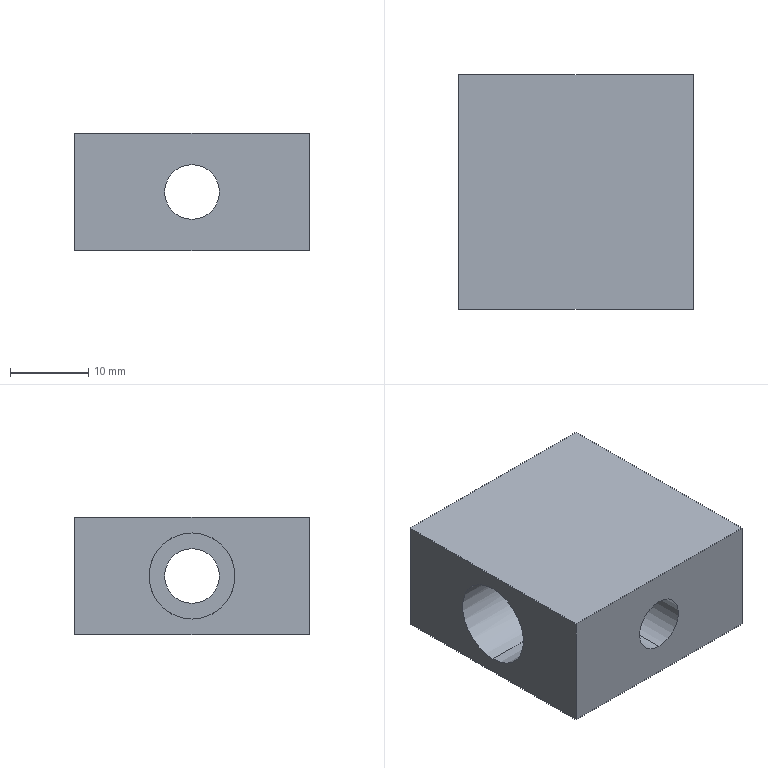Part | SolidWorks | features BaseBody 1 | 1 solid | 20 faces | box 30 x 30 x 15 mm | volume 9251 mm3 | cylinder 12 | plane 8 | commonest cylinder face diameters 11 x8 7 x4
STEP:
#1=CARTESIAN_POINT('',(30.,15.,4.));
#2=VERTEX_POINT('',#1);
#3=CARTESIAN_POINT('',(30.,15.,11.));
#4=VERTEX_POINT('',#3);
#5=CARTESIAN_POINT('',(30.,15.,7.5));
#6=DIRECTION('',(-1.,0.,0.));
#7=DIRECTION('',(0.,0.,1.));
#8=AXIS2_PLACEMENT_3D('',#5,#6,#7);
#9=CIRCLE('',#8,3.5);
#10=EDGE_CURVE('',#2,#4,#9,.T.);
#11=ORIENTED_EDGE('',*,*,#10,.F.);
#12=CARTESIAN_POINT('',(25.,15.,4.));
#13=VERTEX_POINT('',#12);
#14=CARTESIAN_POINT('',(0.,15.,4.));
#15=DIRECTION('',(-1.,0.,0.));
#16=VECTOR('',#15,1000.);
#17=LINE('',#14,#16);
#18=EDGE_CURVE('',#2,#13,#17,.T.);
#19=ORIENTED_EDGE('',*,*,#18,.T.);
#20=CARTESIAN_POINT('',(25.,15.,11.));
#21=VERTEX_POINT('',#20);
#22=CARTESIAN_POINT('',(25.,15.,7.5));
#23=DIRECTION('',(-1.,0.,0.));
#24=DIRECTION('',(0.,0.,1.));
#25=AXIS2_PLACEMENT_3D('',#22,#23,#24);
#26=CIRCLE('',#25,3.5);
#27=EDGE_CURVE('',#13,#21,#26,.T.);
#28=ORIENTED_EDGE('',*,*,#27,.T.);
#29=CARTESIAN_POINT('',(0.,15.,11.));
#30=DIRECTION('',(-1.,0.,0.));
#31=VECTOR('',#30,1000.);
#32=LINE('',#29,#31);
#33=EDGE_CURVE('',#4,#21,#32,.T.);
#34=ORIENTED_EDGE('',*,*,#33,.F.);
#35=EDGE_LOOP('',(#11,#19,#28,#34));
#36=FACE_OUTER_BOUND('',#35,.T.);
#37=CARTESIAN_POINT('',(0.,15.,7.5));
#38=DIRECTION('',(-1.,0.,0.));
#39=DIRECTION('',(0.,0.,1.));
#40=AXIS2_PLACEMENT_3D('',#37,#38,#39);
#41=CYLINDRICAL_SURFACE('',#40,3.5);
#42=ADVANCED_FACE('',(#36),#41,.F.);
#43=CARTESIAN_POINT('',(25.,15.,2.));
#44=VERTEX_POINT('',#43);
#45=CARTESIAN_POINT('',(25.,15.,13.));
#46=VERTEX_POINT('',#45);
#47=CARTESIAN_POINT('',(25.,15.,7.5));
#48=DIRECTION('',(-1.,0.,0.));
#49=DIRECTION('',(0.,0.,1.));
#50=AXIS2_PLACEMENT_3D('',#47,#48,#49);
#51=CIRCLE('',#50,5.5);
#52=EDGE_CURVE('',#44,#46,#51,.T.);
#53=ORIENTED_EDGE('',*,*,#52,.F.);
#54=CARTESIAN_POINT('',(15.,15.,2.));
#55=VERTEX_POINT('',#54);
#56=CARTESIAN_POINT('',(0.,15.,2.));
#57=DIRECTION('',(-1.,0.,0.));
#58=VECTOR('',#57,1000.);
#59=LINE('',#56,#58);
#60=EDGE_CURVE('',#44,#55,#59,.T.);
#61=ORIENTED_EDGE('',*,*,#60,.T.);
#62=CARTESIAN_POINT('',(15.,15.,13.));
#63=VERTEX_POINT('',#62);
#64=CARTESIAN_POINT('',(15.,15.,13.));
#65=CARTESIAN_POINT('',(26.,4.,13.));
#66=CARTESIAN_POINT('',(26.,4.,2.));
#67=CARTESIAN_POINT('',(15.,15.,2.));
#68=(BOUNDED_CURVE()B_SPLINE_CURVE(3,(#64,#65,#66,#67),.UNSPECIFIED.,.F.,.F.)B_SPLINE_CURVE_WITH_KNOTS((4,4),(1.571,4.712),.UNSPECIFIED.)CURVE()GEOMETRIC_REPRESENTATION_ITEM()RATIONAL_B_SPLINE_CURVE((1.,0.3333,0.3333,1.))REPRESENTATION_ITEM(''));
#69=EDGE_CURVE('',#63,#55,#68,.T.);
#70=ORIENTED_EDGE('',*,*,#69,.F.);
#71=CARTESIAN_POINT('',(0.,15.,13.));
#72=DIRECTION('',(-1.,0.,0.));
#73=VECTOR('',#72,1000.);
#74=LINE('',#71,#73);
#75=EDGE_CURVE('',#46,#63,#74,.T.);
#76=ORIENTED_EDGE('',*,*,#75,.F.);
#77=EDGE_LOOP('',(#53,#61,#70,#76));
#78=FACE_OUTER_BOUND('',#77,.T.);
#79=CARTESIAN_POINT('',(0.,15.,7.5));
#80=DIRECTION('',(-1.,0.,0.));
#81=DIRECTION('',(0.,0.,1.));
#82=AXIS2_PLACEMENT_3D('',#79,#80,#81);
#83=CYLINDRICAL_SURFACE('',#82,5.5);
#84=ADVANCED_FACE('',(#78),#83,.F.);
#85=CARTESIAN_POINT('',(15.,15.,2.));
#86=CARTESIAN_POINT('',(4.,4.,2.));
#87=CARTESIAN_POINT('',(4.,4.,13.));
#88=CARTESIAN_POINT('',(15.,15.,13.));
#89=(BOUNDED_CURVE()B_SPLINE_CURVE(3,(#85,#86,#87,#88),.UNSPECIFIED.,.F.,.F.)B_SPLINE_CURVE_WITH_KNOTS((4,4),(1.571,4.712),.UNSPECIFIED.)CURVE()GEOMETRIC_REPRESENTATION_ITEM()RATIONAL_B_SPLINE_CURVE((1.,0.3333,0.3333,1.))REPRESENTATION_ITEM(''));
#90=EDGE_CURVE('',#55,#63,#89,.T.);
#91=ORIENTED_EDGE('',*,*,#90,.F.);
#92=CARTESIAN_POINT('',(0.,15.,2.));
#93=VERTEX_POINT('',#92);
#94=CARTESIAN_POINT('',(0.,15.,2.));
#95=DIRECTION('',(-1.,0.,0.));
#96=VECTOR('',#95,1000.);
#97=LINE('',#94,#96);
#98=EDGE_CURVE('',#55,#93,#97,.T.);
#99=ORIENTED_EDGE('',*,*,#98,.T.);
#100=CARTESIAN_POINT('',(0.,15.,13.));
#101=VERTEX_POINT('',#100);
#102=CARTESIAN_POINT('',(0.,15.,7.5));
#103=DIRECTION('',(-1.,0.,0.));
#104=DIRECTION('',(0.,0.,1.));
#105=AXIS2_PLACEMENT_3D('',#102,#103,#104);
#106=CIRCLE('',#105,5.5);
#107=EDGE_CURVE('',#93,#101,#106,.T.);
#108=ORIENTED_EDGE('',*,*,#107,.T.);
#109=CARTESIAN_POINT('',(0.,15.,13.));
#110=DIRECTION('',(-1.,0.,0.));
#111=VECTOR('',#110,1000.);
#112=LINE('',#109,#111);
#113=EDGE_CURVE('',#63,#101,#112,.T.);
#114=ORIENTED_EDGE('',*,*,#113,.F.);
#115=EDGE_LOOP('',(#91,#99,#108,#114));
#116=FACE_OUTER_BOUND('',#115,.T.);
#117=CARTESIAN_POINT('',(0.,15.,7.5));
#118=DIRECTION('',(-1.,0.,0.));
#119=DIRECTION('',(0.,0.,1.));
#120=AXIS2_PLACEMENT_3D('',#117,#118,#119);
#121=CYLINDRICAL_SURFACE('',#120,5.5);
#122=ADVANCED_FACE('',(#116),#121,.F.);
#123=CARTESIAN_POINT('',(15.,5.,2.));
#124=VERTEX_POINT('',#123);
#125=CARTESIAN_POINT('',(15.,5.,13.));
#126=VERTEX_POINT('',#125);
#127=CARTESIAN_POINT('',(15.,5.,7.5));
#128=DIRECTION('',(0.,1.,0.));
#129=DIRECTION('',(0.,0.,1.));
#130=AXIS2_PLACEMENT_3D('',#127,#128,#129);
#131=CIRCLE('',#130,5.5);
#132=EDGE_CURVE('',#124,#126,#131,.T.);
#133=ORIENTED_EDGE('',*,*,#132,.F.);
#134=CARTESIAN_POINT('',(15.,30.,2.));
#135=DIRECTION('',(0.,1.,0.));
#136=VECTOR('',#135,1000.);
#137=LINE('',#134,#136);
#138=EDGE_CURVE('',#124,#55,#137,.T.);
#139=ORIENTED_EDGE('',*,*,#138,.T.);
#140=ORIENTED_EDGE('',*,*,#90,.T.);
#141=CARTESIAN_POINT('',(15.,30.,13.));
#142=DIRECTION('',(0.,1.,0.));
#143=VECTOR('',#142,1000.);
#144=LINE('',#141,#143);
#145=EDGE_CURVE('',#126,#63,#144,.T.);
#146=ORIENTED_EDGE('',*,*,#145,.F.);
#147=EDGE_LOOP('',(#133,#139,#140,#146));
#148=FACE_OUTER_BOUND('',#147,.T.);
#149=CARTESIAN_POINT('',(15.,30.,7.5));
#150=DIRECTION('',(0.,1.,0.));
#151=DIRECTION('',(0.,0.,1.));
#152=AXIS2_PLACEMENT_3D('',#149,#150,#151);
#153=CYLINDRICAL_SURFACE('',#152,5.5);
#154=ADVANCED_FACE('',(#148),#153,.F.);
#155=CARTESIAN_POINT('',(15.,0.,4.));
#156=VERTEX_POINT('',#155);
#157=CARTESIAN_POINT('',(15.,0.,11.));
#158=VERTEX_POINT('',#157);
#159=CARTESIAN_POINT('',(15.,0.,7.5));
#160=DIRECTION('',(0.,1.,0.));
#161=DIRECTION('',(0.,0.,1.));
#162=AXIS2_PLACEMENT_3D('',#159,#160,#161);
#163=CIRCLE('',#162,3.5);
#164=EDGE_CURVE('',#156,#158,#163,.T.);
#165=ORIENTED_EDGE('',*,*,#164,.F.);
#166=CARTESIAN_POINT('',(15.,5.,4.));
#167=VERTEX_POINT('',#166);
#168=CARTESIAN_POINT('',(15.,30.,4.));
#169=DIRECTION('',(0.,1.,0.));
#170=VECTOR('',#169,1000.);
#171=LINE('',#168,#170);
#172=EDGE_CURVE('',#156,#167,#171,.T.);
#173=ORIENTED_EDGE('',*,*,#172,.T.);
#174=CARTESIAN_POINT('',(15.,5.,11.));
#175=VERTEX_POINT('',#174);
#176=CARTESIAN_POINT('',(15.,5.,7.5));
#177=DIRECTION('',(0.,1.,0.));
#178=DIRECTION('',(0.,0.,1.));
#179=AXIS2_PLACEMENT_3D('',#176,#177,#178);
#180=CIRCLE('',#179,3.5);
#181=EDGE_CURVE('',#167,#175,#180,.T.);
#182=ORIENTED_EDGE('',*,*,#181,.T.);
#183=CARTESIAN_POINT('',(15.,30.,11.));
#184=DIRECTION('',(0.,1.,0.));
#185=VECTOR('',#184,1000.);
#186=LINE('',#183,#185);
#187=EDGE_CURVE('',#158,#175,#186,.T.);
#188=ORIENTED_EDGE('',*,*,#187,.F.);
#189=EDGE_LOOP('',(#165,#173,#182,#188));
#190=FACE_OUTER_BOUND('',#189,.T.);
#191=CARTESIAN_POINT('',(15.,30.,7.5));
#192=DIRECTION('',(0.,1.,0.));
#193=DIRECTION('',(0.,0.,1.));
#194=AXIS2_PLACEMENT_3D('',#191,#192,#193);
#195=CYLINDRICAL_SURFACE('',#194,3.5);
#196=ADVANCED_FACE('',(#190),#195,.F.);
#197=CARTESIAN_POINT('',(15.,15.,13.));
#198=CARTESIAN_POINT('',(4.,26.,13.));
#199=CARTESIAN_POINT('',(4.,26.,2.));
#200=CARTESIAN_POINT('',(15.,15.,2.));
#201=(BOUNDED_CURVE()B_SPLINE_CURVE(3,(#197,#198,#199,#200),.UNSPECIFIED.,.F.,.F.)B_SPLINE_CURVE_WITH_KNOTS((4,4),(4.712,7.854),.UNSPECIFIED.)CURVE()GEOMETRIC_REPRESENTATION_ITEM()RATIONAL_B_SPLINE_CURVE((1.,0.3333,0.3333,1.))REPRESENTATION_ITEM(''));
#202=EDGE_CURVE('',#63,#55,#201,.T.);
#203=ORIENTED_EDGE('',*,*,#202,.T.);
#204=CARTESIAN_POINT('',(15.,30.,2.));
#205=VERTEX_POINT('',#204);
#206=CARTESIAN_POINT('',(15.,30.,2.));
#207=DIRECTION('',(0.,1.,0.));
#208=VECTOR('',#207,1000.);
#209=LINE('',#206,#208);
#210=EDGE_CURVE('',#55,#205,#209,.T.);
#211=ORIENTED_EDGE('',*,*,#210,.T.);
#212=CARTESIAN_POINT('',(15.,30.,13.));
#213=VERTEX_POINT('',#212);
#214=CARTESIAN_POINT('',(15.,30.,7.5));
#215=DIRECTION('',(0.,1.,0.));
#216=DIRECTION('',(0.,0.,1.));
#217=AXIS2_PLACEMENT_3D('',#214,#215,#216);
#218=CIRCLE('',#217,5.5);
#219=EDGE_CURVE('',#205,#213,#218,.T.);
#220=ORIENTED_EDGE('',*,*,#219,.T.);
#221=CARTESIAN_POINT('',(15.,30.,13.));
#222=DIRECTION('',(0.,1.,0.));
#223=VECTOR('',#222,1000.);
#224=LINE('',#221,#223);
#225=EDGE_CURVE('',#63,#213,#224,.T.);
#226=ORIENTED_EDGE('',*,*,#225,.F.);
#227=EDGE_LOOP('',(#203,#211,#220,#226));
#228=FACE_OUTER_BOUND('',#227,.T.);
#229=CARTESIAN_POINT('',(15.,30.,7.5));
#230=DIRECTION('',(0.,1.,0.));
#231=DIRECTION('',(0.,0.,1.));
#232=AXIS2_PLACEMENT_3D('',#229,#230,#231);
#233=CYLINDRICAL_SURFACE('',#232,5.5);
#234=ADVANCED_FACE('',(#228),#233,.F.);
#235=CARTESIAN_POINT('',(25.,15.,7.5));
#236=DIRECTION('',(-1.,0.,0.));
#237=DIRECTION('',(0.,0.,1.));
#238=AXIS2_PLACEMENT_3D('',#235,#236,#237);
#239=CIRCLE('',#238,3.5);
#240=EDGE_CURVE('',#21,#13,#239,.T.);
#241=ORIENTED_EDGE('',*,*,#240,.F.);
#242=ORIENTED_EDGE('',*,*,#27,.F.);
#243=EDGE_LOOP('',(#241,#242));
#244=FACE_BOUND('',#243,.T.);
#245=CARTESIAN_POINT('',(25.,15.,7.5));
#246=DIRECTION('',(-1.,0.,0.));
#247=DIRECTION('',(0.,0.,1.));
#248=AXIS2_PLACEMENT_3D('',#245,#246,#247);
#249=CIRCLE('',#248,5.5);
#250=EDGE_CURVE('',#46,#44,#249,.T.);
#251=ORIENTED_EDGE('',*,*,#250,.T.);
#252=ORIENTED_EDGE('',*,*,#52,.T.);
#253=EDGE_LOOP('',(#251,#252));
#254=FACE_OUTER_BOUND('',#253,.T.);
#255=CARTESIAN_POINT('',(25.,18.5,7.5));
#256=DIRECTION('',(1.,0.,0.));
#257=DIRECTION('',(0.,1.,0.));
#258=AXIS2_PLACEMENT_3D('',#255,#256,#257);
#259=PLANE('',#258);
#260=ADVANCED_FACE('',(#244,#254),#259,.F.);
#261=CARTESIAN_POINT('',(15.,5.,7.5));
#262=DIRECTION('',(0.,1.,0.));
#263=DIRECTION('',(0.,0.,1.));
#264=AXIS2_PLACEMENT_3D('',#261,#262,#263);
#265=CIRCLE('',#264,3.5);
#266=EDGE_CURVE('',#175,#167,#265,.T.);
#267=ORIENTED_EDGE('',*,*,#266,.F.);
#268=ORIENTED_EDGE('',*,*,#181,.F.);
#269=EDGE_LOOP('',(#267,#268));
#270=FACE_BOUND('',#269,.T.);
#271=CARTESIAN_POINT('',(15.,5.,7.5));
#272=DIRECTION('',(0.,1.,0.));
#273=DIRECTION('',(0.,0.,1.));
#274=AXIS2_PLACEMENT_3D('',#271,#272,#273);
#275=CIRCLE('',#274,5.5);
#276=EDGE_CURVE('',#126,#124,#275,.T.);
#277=ORIENTED_EDGE('',*,*,#276,.T.);
#278=ORIENTED_EDGE('',*,*,#132,.T.);
#279=EDGE_LOOP('',(#277,#278));
#280=FACE_OUTER_BOUND('',#279,.T.);
#281=CARTESIAN_POINT('',(18.5,5.,7.5));
#282=DIRECTION('',(0.,-1.,0.));
#283=DIRECTION('',(0.,0.,-1.));
#284=AXIS2_PLACEMENT_3D('',#281,#282,#283);
#285=PLANE('',#284);
#286=ADVANCED_FACE('',(#270,#280),#285,.F.);
#287=CARTESIAN_POINT('',(0.,30.,0.));
#288=VERTEX_POINT('',#287);
#289=CARTESIAN_POINT('',(0.,0.,0.));
#290=VERTEX_POINT('',#289);
#291=CARTESIAN_POINT('',(0.,0.,0.));
#292=DIRECTION('',(0.,-1.,0.));
#293=VECTOR('',#292,1000.);
#294=LINE('',#291,#293);
#295=EDGE_CURVE('',#288,#290,#294,.T.);
#296=ORIENTED_EDGE('',*,*,#295,.F.);
#297=CARTESIAN_POINT('',(30.,30.,0.));
#298=VERTEX_POINT('',#297);
#299=CARTESIAN_POINT('',(0.,30.,0.));
#300=DIRECTION('',(-1.,0.,0.));
#301=VECTOR('',#300,1000.);
#302=LINE('',#299,#301);
#303=EDGE_CURVE('',#298,#288,#302,.T.);
#304=ORIENTED_EDGE('',*,*,#303,.F.);
#305=CARTESIAN_POINT('',(30.,0.,0.));
#306=VERTEX_POINT('',#305);
#307=CARTESIAN_POINT('',(30.,0.,0.));
#308=DIRECTION('',(0.,1.,0.));
#309=VECTOR('',#308,1000.);
#310=LINE('',#307,#309);
#311=EDGE_CURVE('',#306,#298,#310,.T.);
#312=ORIENTED_EDGE('',*,*,#311,.F.);
#313=CARTESIAN_POINT('',(0.,0.,0.));
#314=DIRECTION('',(1.,0.,0.));
#315=VECTOR('',#314,1000.);
#316=LINE('',#313,#315);
#317=EDGE_CURVE('',#290,#306,#316,.T.);
#318=ORIENTED_EDGE('',*,*,#317,.F.);
#319=EDGE_LOOP('',(#296,#304,#312,#318));
#320=FACE_OUTER_BOUND('',#319,.T.);
#321=CARTESIAN_POINT('',(0.,0.,0.));
#322=DIRECTION('',(0.,0.,-1.));
#323=DIRECTION('',(0.,-1.,0.));
#324=AXIS2_PLACEMENT_3D('',#321,#322,#323);
#325=PLANE('',#324);
#326=ADVANCED_FACE('',(#320),#325,.T.);
#327=CARTESIAN_POINT('',(0.,30.,15.));
#328=VERTEX_POINT('',#327);
#329=CARTESIAN_POINT('',(0.,0.,15.));
#330=VERTEX_POINT('',#329);
#331=CARTESIAN_POINT('',(0.,0.,15.));
#332=DIRECTION('',(0.,-1.,0.));
#333=VECTOR('',#332,1000.);
#334=LINE('',#331,#333);
#335=EDGE_CURVE('',#328,#330,#334,.T.);
#336=ORIENTED_EDGE('',*,*,#335,.T.);
#337=CARTESIAN_POINT('',(30.,0.,15.));
#338=VERTEX_POINT('',#337);
#339=CARTESIAN_POINT('',(0.,0.,15.));
#340=DIRECTION('',(1.,0.,0.));
#341=VECTOR('',#340,1000.);
#342=LINE('',#339,#341);
#343=EDGE_CURVE('',#330,#338,#342,.T.);
#344=ORIENTED_EDGE('',*,*,#343,.T.);
#345=CARTESIAN_POINT('',(30.,30.,15.));
#346=VERTEX_POINT('',#345);
#347=CARTESIAN_POINT('',(30.,0.,15.));
#348=DIRECTION('',(0.,1.,0.));
#349=VECTOR('',#348,1000.);
#350=LINE('',#347,#349);
#351=EDGE_CURVE('',#338,#346,#350,.T.);
#352=ORIENTED_EDGE('',*,*,#351,.T.);
#353=CARTESIAN_POINT('',(0.,30.,15.));
#354=DIRECTION('',(-1.,0.,0.));
#355=VECTOR('',#354,1000.);
#356=LINE('',#353,#355);
#357=EDGE_CURVE('',#346,#328,#356,.T.);
#358=ORIENTED_EDGE('',*,*,#357,.T.);
#359=EDGE_LOOP('',(#336,#344,#352,#358));
#360=FACE_OUTER_BOUND('',#359,.T.);
#361=CARTESIAN_POINT('',(0.,0.,15.));
#362=DIRECTION('',(0.,0.,-1.));
#363=DIRECTION('',(0.,-1.,0.));
#364=AXIS2_PLACEMENT_3D('',#361,#362,#363);
#365=PLANE('',#364);
#366=ADVANCED_FACE('',(#360),#365,.F.);
#367=CARTESIAN_POINT('',(15.,30.,7.5));
#368=DIRECTION('',(0.,1.,0.));
#369=DIRECTION('',(0.,0.,1.));
#370=AXIS2_PLACEMENT_3D('',#367,#368,#369);
#371=CIRCLE('',#370,5.5);
#372=EDGE_CURVE('',#213,#205,#371,.T.);
#373=ORIENTED_EDGE('',*,*,#372,.F.);
#374=ORIENTED_EDGE('',*,*,#219,.F.);
#375=EDGE_LOOP('',(#373,#374));
#376=FACE_BOUND('',#375,.T.);
#377=ORIENTED_EDGE('',*,*,#303,.T.);
#378=CARTESIAN_POINT('',(0.,30.,15.));
#379=DIRECTION('',(0.,0.,-1.));
#380=VECTOR('',#379,1000.);
#381=LINE('',#378,#380);
#382=EDGE_CURVE('',#328,#288,#381,.T.);
#383=ORIENTED_EDGE('',*,*,#382,.F.);
#384=ORIENTED_EDGE('',*,*,#357,.F.);
#385=CARTESIAN_POINT('',(30.,30.,15.));
#386=DIRECTION('',(0.,0.,-1.));
#387=VECTOR('',#386,1000.);
#388=LINE('',#385,#387);
#389=EDGE_CURVE('',#346,#298,#388,.T.);
#390=ORIENTED_EDGE('',*,*,#389,.T.);
#391=EDGE_LOOP('',(#377,#383,#384,#390));
#392=FACE_OUTER_BOUND('',#391,.T.);
#393=CARTESIAN_POINT('',(0.,30.,15.));
#394=DIRECTION('',(0.,-1.,0.));
#395=DIRECTION('',(0.,0.,-1.));
#396=AXIS2_PLACEMENT_3D('',#393,#394,#395);
#397=PLANE('',#396);
#398=ADVANCED_FACE('',(#376,#392),#397,.F.);
#399=CARTESIAN_POINT('',(30.,15.,7.5));
#400=DIRECTION('',(-1.,0.,0.));
#401=DIRECTION('',(0.,0.,1.));
#402=AXIS2_PLACEMENT_3D('',#399,#400,#401);
#403=CIRCLE('',#402,3.5);
#404=EDGE_CURVE('',#4,#2,#403,.T.);
#405=ORIENTED_EDGE('',*,*,#404,.T.);
#406=ORIENTED_EDGE('',*,*,#10,.T.);
#407=EDGE_LOOP('',(#405,#406));
#408=FACE_BOUND('',#407,.T.);
#409=ORIENTED_EDGE('',*,*,#311,.T.);
#410=ORIENTED_EDGE('',*,*,#389,.F.);
#411=ORIENTED_EDGE('',*,*,#351,.F.);
#412=CARTESIAN_POINT('',(30.,0.,15.));
#413=DIRECTION('',(0.,0.,-1.));
#414=VECTOR('',#413,1000.);
#415=LINE('',#412,#414);
#416=EDGE_CURVE('',#338,#306,#415,.T.);
#417=ORIENTED_EDGE('',*,*,#416,.T.);
#418=EDGE_LOOP('',(#409,#410,#411,#417));
#419=FACE_OUTER_BOUND('',#418,.T.);
#420=CARTESIAN_POINT('',(30.,0.,15.));
#421=DIRECTION('',(-1.,0.,0.));
#422=DIRECTION('',(0.,0.,1.));
#423=AXIS2_PLACEMENT_3D('',#420,#421,#422);
#424=PLANE('',#423);
#425=ADVANCED_FACE('',(#408,#419),#424,.F.);
#426=CARTESIAN_POINT('',(15.,0.,7.5));
#427=DIRECTION('',(0.,1.,0.));
#428=DIRECTION('',(0.,0.,1.));
#429=AXIS2_PLACEMENT_3D('',#426,#427,#428);
#430=CIRCLE('',#429,3.5);
#431=EDGE_CURVE('',#158,#156,#430,.T.);
#432=ORIENTED_EDGE('',*,*,#431,.T.);
#433=ORIENTED_EDGE('',*,*,#164,.T.);
#434=EDGE_LOOP('',(#432,#433));
#435=FACE_BOUND('',#434,.T.);
#436=ORIENTED_EDGE('',*,*,#317,.T.);
#437=ORIENTED_EDGE('',*,*,#416,.F.);
#438=ORIENTED_EDGE('',*,*,#343,.F.);
#439=CARTESIAN_POINT('',(0.,0.,15.));
#440=DIRECTION('',(0.,0.,-1.));
#441=VECTOR('',#440,1000.);
#442=LINE('',#439,#441);
#443=EDGE_CURVE('',#330,#290,#442,.T.);
#444=ORIENTED_EDGE('',*,*,#443,.T.);
#445=EDGE_LOOP('',(#436,#437,#438,#444));
#446=FACE_OUTER_BOUND('',#445,.T.);
#447=CARTESIAN_POINT('',(0.,0.,15.));
#448=DIRECTION('',(0.,1.,0.));
#449=DIRECTION('',(1.,0.,0.));
#450=AXIS2_PLACEMENT_3D('',#447,#448,#449);
#451=PLANE('',#450);
#452=ADVANCED_FACE('',(#435,#446),#451,.F.);
#453=CARTESIAN_POINT('',(0.,15.,7.5));
#454=DIRECTION('',(-1.,0.,0.));
#455=DIRECTION('',(0.,0.,1.));
#456=AXIS2_PLACEMENT_3D('',#453,#454,#455);
#457=CIRCLE('',#456,5.5);
#458=EDGE_CURVE('',#101,#93,#457,.T.);
#459=ORIENTED_EDGE('',*,*,#458,.F.);
#460=ORIENTED_EDGE('',*,*,#107,.F.);
#461=EDGE_LOOP('',(#459,#460));
#462=FACE_BOUND('',#461,.T.);
#463=ORIENTED_EDGE('',*,*,#295,.T.);
#464=ORIENTED_EDGE('',*,*,#443,.F.);
#465=ORIENTED_EDGE('',*,*,#335,.F.);
#466=ORIENTED_EDGE('',*,*,#382,.T.);
#467=EDGE_LOOP('',(#463,#464,#465,#466));
#468=FACE_OUTER_BOUND('',#467,.T.);
#469=CARTESIAN_POINT('',(0.,0.,15.));
#470=DIRECTION('',(1.,0.,0.));
#471=DIRECTION('',(0.,1.,0.));
#472=AXIS2_PLACEMENT_3D('',#469,#470,#471);
#473=PLANE('',#472);
#474=ADVANCED_FACE('',(#462,#468),#473,.F.);
#475=ORIENTED_EDGE('',*,*,#210,.F.);
#476=CARTESIAN_POINT('',(15.,15.,2.));
#477=CARTESIAN_POINT('',(26.,26.,2.));
#478=CARTESIAN_POINT('',(26.,26.,13.));
#479=CARTESIAN_POINT('',(15.,15.,13.));
#480=(BOUNDED_CURVE()B_SPLINE_CURVE(3,(#476,#477,#478,#479),.UNSPECIFIED.,.F.,.T.)B_SPLINE_CURVE_WITH_KNOTS((4,4),(4.712,7.854),.UNSPECIFIED.)CURVE()GEOMETRIC_REPRESENTATION_ITEM()RATIONAL_B_SPLINE_CURVE((1.,0.3333,0.3333,1.))REPRESENTATION_ITEM(''));
#481=EDGE_CURVE('',#55,#63,#480,.T.);
#482=ORIENTED_EDGE('',*,*,#481,.T.);
#483=ORIENTED_EDGE('',*,*,#225,.T.);
#484=ORIENTED_EDGE('',*,*,#372,.T.);
#485=EDGE_LOOP('',(#475,#482,#483,#484));
#486=FACE_OUTER_BOUND('',#485,.T.);
#487=CARTESIAN_POINT('',(15.,30.,7.5));
#488=DIRECTION('',(0.,1.,0.));
#489=DIRECTION('',(0.,0.,1.));
#490=AXIS2_PLACEMENT_3D('',#487,#488,#489);
#491=CYLINDRICAL_SURFACE('',#490,5.5);
#492=ADVANCED_FACE('',(#486),#491,.F.);
#493=ORIENTED_EDGE('',*,*,#172,.F.);
#494=ORIENTED_EDGE('',*,*,#431,.F.);
#495=ORIENTED_EDGE('',*,*,#187,.T.);
#496=ORIENTED_EDGE('',*,*,#266,.T.);
#497=EDGE_LOOP('',(#493,#494,#495,#496));
#498=FACE_OUTER_BOUND('',#497,.T.);
#499=CARTESIAN_POINT('',(15.,30.,7.5));
#500=DIRECTION('',(0.,1.,0.));
#501=DIRECTION('',(0.,0.,1.));
#502=AXIS2_PLACEMENT_3D('',#499,#500,#501);
#503=CYLINDRICAL_SURFACE('',#502,3.5);
#504=ADVANCED_FACE('',(#498),#503,.F.);
#505=ORIENTED_EDGE('',*,*,#138,.F.);
#506=ORIENTED_EDGE('',*,*,#276,.F.);
#507=ORIENTED_EDGE('',*,*,#145,.T.);
#508=ORIENTED_EDGE('',*,*,#69,.T.);
#509=EDGE_LOOP('',(#505,#506,#507,#508));
#510=FACE_OUTER_BOUND('',#509,.T.);
#511=CARTESIAN_POINT('',(15.,30.,7.5));
#512=DIRECTION('',(0.,1.,0.));
#513=DIRECTION('',(0.,0.,1.));
#514=AXIS2_PLACEMENT_3D('',#511,#512,#513);
#515=CYLINDRICAL_SURFACE('',#514,5.5);
#516=ADVANCED_FACE('',(#510),#515,.F.);
#517=ORIENTED_EDGE('',*,*,#98,.F.);
#518=ORIENTED_EDGE('',*,*,#202,.F.);
#519=ORIENTED_EDGE('',*,*,#113,.T.);
#520=ORIENTED_EDGE('',*,*,#458,.T.);
#521=EDGE_LOOP('',(#517,#518,#519,#520));
#522=FACE_OUTER_BOUND('',#521,.T.);
#523=CARTESIAN_POINT('',(0.,15.,7.5));
#524=DIRECTION('',(-1.,0.,0.));
#525=DIRECTION('',(0.,0.,1.));
#526=AXIS2_PLACEMENT_3D('',#523,#524,#525);
#527=CYLINDRICAL_SURFACE('',#526,5.5);
#528=ADVANCED_FACE('',(#522),#527,.F.);
#529=ORIENTED_EDGE('',*,*,#60,.F.);
#530=ORIENTED_EDGE('',*,*,#250,.F.);
#531=ORIENTED_EDGE('',*,*,#75,.T.);
#532=ORIENTED_EDGE('',*,*,#481,.F.);
#533=EDGE_LOOP('',(#529,#530,#531,#532));
#534=FACE_OUTER_BOUND('',#533,.T.);
#535=CARTESIAN_POINT('',(0.,15.,7.5));
#536=DIRECTION('',(-1.,0.,0.));
#537=DIRECTION('',(0.,0.,1.));
#538=AXIS2_PLACEMENT_3D('',#535,#536,#537);
#539=CYLINDRICAL_SURFACE('',#538,5.5);
#540=ADVANCED_FACE('',(#534),#539,.F.);
#541=ORIENTED_EDGE('',*,*,#18,.F.);
#542=ORIENTED_EDGE('',*,*,#404,.F.);
#543=ORIENTED_EDGE('',*,*,#33,.T.);
#544=ORIENTED_EDGE('',*,*,#240,.T.);
#545=EDGE_LOOP('',(#541,#542,#543,#544));
#546=FACE_OUTER_BOUND('',#545,.T.);
#547=CARTESIAN_POINT('',(0.,15.,7.5));
#548=DIRECTION('',(-1.,0.,0.));
#549=DIRECTION('',(0.,0.,1.));
#550=AXIS2_PLACEMENT_3D('',#547,#548,#549);
#551=CYLINDRICAL_SURFACE('',#550,3.5);
#552=ADVANCED_FACE('',(#546),#551,.F.);
#553=CLOSED_SHELL('',(#42,#84,#122,#154,#196,#234,#260,#286,#326,#366,#398,#425,#452,#474,#492,#504,#516,#528,#540,#552));
#554=MANIFOLD_SOLID_BREP('',#553);
#555=CARTESIAN_POINT('',(0.,0.,0.));
#556=DIRECTION('',(0.,0.,1.));
#557=DIRECTION('',(1.,0.,0.));
#558=AXIS2_PLACEMENT_3D('',#555,#556,#557);
#559=(LENGTH_UNIT()NAMED_UNIT(*)SI_UNIT(.MILLI.,.METRE.));
#560=UNCERTAINTY_MEASURE_WITH_UNIT(LENGTH_MEASURE(0.00001),#559,'','');
#561=(NAMED_UNIT(*)PLANE_ANGLE_UNIT()SI_UNIT($,.RADIAN.));
#562=(NAMED_UNIT(*)SI_UNIT($,.STERADIAN.)SOLID_ANGLE_UNIT());
#563=(GEOMETRIC_REPRESENTATION_CONTEXT(3)GLOBAL_UNCERTAINTY_ASSIGNED_CONTEXT((#560))GLOBAL_UNIT_ASSIGNED_CONTEXT((#559,#561,#562))REPRESENTATION_CONTEXT('',''));
#564=ADVANCED_BREP_SHAPE_REPRESENTATION('',(#554,#558),#563);